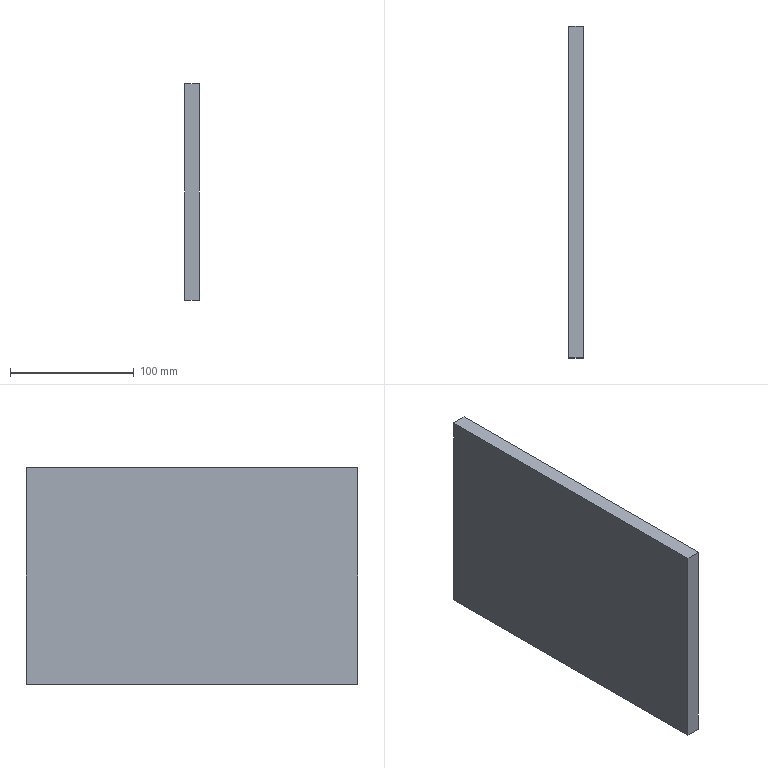Part | SolidWorks | features Extrusion 1 | 1 solid | 6 faces | box 12 x 268 x 175 mm | volume 562800 mm3 | plane 6
STEP:
#1=CARTESIAN_POINT('',(0.,268.,0.));
#2=VERTEX_POINT('',#1);
#3=CARTESIAN_POINT('',(0.,0.,0.));
#4=VERTEX_POINT('',#3);
#5=CARTESIAN_POINT('',(0.,0.,0.));
#6=DIRECTION('',(0.,-1.,0.));
#7=VECTOR('',#6,1000.);
#8=LINE('',#5,#7);
#9=EDGE_CURVE('',#2,#4,#8,.T.);
#10=ORIENTED_EDGE('',*,*,#9,.T.);
#11=CARTESIAN_POINT('',(12.,0.,0.));
#12=VERTEX_POINT('',#11);
#13=CARTESIAN_POINT('',(12.,0.,0.));
#14=DIRECTION('',(-1.,0.,0.));
#15=VECTOR('',#14,1000.);
#16=LINE('',#13,#15);
#17=EDGE_CURVE('',#12,#4,#16,.T.);
#18=ORIENTED_EDGE('',*,*,#17,.F.);
#19=CARTESIAN_POINT('',(12.,268.,0.));
#20=VERTEX_POINT('',#19);
#21=CARTESIAN_POINT('',(12.,0.,0.));
#22=DIRECTION('',(0.,-1.,0.));
#23=VECTOR('',#22,1000.);
#24=LINE('',#21,#23);
#25=EDGE_CURVE('',#20,#12,#24,.T.);
#26=ORIENTED_EDGE('',*,*,#25,.F.);
#27=CARTESIAN_POINT('',(12.,268.,0.));
#28=DIRECTION('',(-1.,0.,0.));
#29=VECTOR('',#28,1000.);
#30=LINE('',#27,#29);
#31=EDGE_CURVE('',#20,#2,#30,.T.);
#32=ORIENTED_EDGE('',*,*,#31,.T.);
#33=EDGE_LOOP('',(#10,#18,#26,#32));
#34=FACE_OUTER_BOUND('',#33,.T.);
#35=CARTESIAN_POINT('',(12.,0.,0.));
#36=DIRECTION('',(0.,0.,-1.));
#37=DIRECTION('',(-1.,0.,0.));
#38=AXIS2_PLACEMENT_3D('',#35,#36,#37);
#39=PLANE('',#38);
#40=ADVANCED_FACE('',(#34),#39,.F.);
#41=CARTESIAN_POINT('',(0.,0.,-175.));
#42=VERTEX_POINT('',#41);
#43=CARTESIAN_POINT('',(0.,0.,0.));
#44=DIRECTION('',(0.,0.,-1.));
#45=VECTOR('',#44,1000.);
#46=LINE('',#43,#45);
#47=EDGE_CURVE('',#4,#42,#46,.T.);
#48=ORIENTED_EDGE('',*,*,#47,.T.);
#49=CARTESIAN_POINT('',(12.,0.,-175.));
#50=VERTEX_POINT('',#49);
#51=CARTESIAN_POINT('',(12.,0.,-175.));
#52=DIRECTION('',(-1.,0.,0.));
#53=VECTOR('',#52,1000.);
#54=LINE('',#51,#53);
#55=EDGE_CURVE('',#50,#42,#54,.T.);
#56=ORIENTED_EDGE('',*,*,#55,.F.);
#57=CARTESIAN_POINT('',(12.,0.,0.));
#58=DIRECTION('',(0.,0.,-1.));
#59=VECTOR('',#58,1000.);
#60=LINE('',#57,#59);
#61=EDGE_CURVE('',#12,#50,#60,.T.);
#62=ORIENTED_EDGE('',*,*,#61,.F.);
#63=ORIENTED_EDGE('',*,*,#17,.T.);
#64=EDGE_LOOP('',(#48,#56,#62,#63));
#65=FACE_OUTER_BOUND('',#64,.T.);
#66=CARTESIAN_POINT('',(12.,0.,0.));
#67=DIRECTION('',(0.,1.,0.));
#68=DIRECTION('',(0.,0.,1.));
#69=AXIS2_PLACEMENT_3D('',#66,#67,#68);
#70=PLANE('',#69);
#71=ADVANCED_FACE('',(#65),#70,.F.);
#72=CARTESIAN_POINT('',(0.,268.,-175.));
#73=VERTEX_POINT('',#72);
#74=CARTESIAN_POINT('',(0.,0.,-175.));
#75=DIRECTION('',(0.,1.,0.));
#76=VECTOR('',#75,1000.);
#77=LINE('',#74,#76);
#78=EDGE_CURVE('',#42,#73,#77,.T.);
#79=ORIENTED_EDGE('',*,*,#78,.T.);
#80=CARTESIAN_POINT('',(12.,268.,-175.));
#81=VERTEX_POINT('',#80);
#82=CARTESIAN_POINT('',(12.,268.,-175.));
#83=DIRECTION('',(-1.,0.,0.));
#84=VECTOR('',#83,1000.);
#85=LINE('',#82,#84);
#86=EDGE_CURVE('',#81,#73,#85,.T.);
#87=ORIENTED_EDGE('',*,*,#86,.F.);
#88=CARTESIAN_POINT('',(12.,0.,-175.));
#89=DIRECTION('',(0.,1.,0.));
#90=VECTOR('',#89,1000.);
#91=LINE('',#88,#90);
#92=EDGE_CURVE('',#50,#81,#91,.T.);
#93=ORIENTED_EDGE('',*,*,#92,.F.);
#94=ORIENTED_EDGE('',*,*,#55,.T.);
#95=EDGE_LOOP('',(#79,#87,#93,#94));
#96=FACE_OUTER_BOUND('',#95,.T.);
#97=CARTESIAN_POINT('',(12.,0.,-175.));
#98=DIRECTION('',(0.,0.,1.));
#99=DIRECTION('',(1.,0.,0.));
#100=AXIS2_PLACEMENT_3D('',#97,#98,#99);
#101=PLANE('',#100);
#102=ADVANCED_FACE('',(#96),#101,.F.);
#103=CARTESIAN_POINT('',(0.,268.,0.));
#104=DIRECTION('',(0.,0.,1.));
#105=VECTOR('',#104,1000.);
#106=LINE('',#103,#105);
#107=EDGE_CURVE('',#73,#2,#106,.T.);
#108=ORIENTED_EDGE('',*,*,#107,.T.);
#109=ORIENTED_EDGE('',*,*,#31,.F.);
#110=CARTESIAN_POINT('',(12.,268.,0.));
#111=DIRECTION('',(0.,0.,1.));
#112=VECTOR('',#111,1000.);
#113=LINE('',#110,#112);
#114=EDGE_CURVE('',#81,#20,#113,.T.);
#115=ORIENTED_EDGE('',*,*,#114,.F.);
#116=ORIENTED_EDGE('',*,*,#86,.T.);
#117=EDGE_LOOP('',(#108,#109,#115,#116));
#118=FACE_OUTER_BOUND('',#117,.T.);
#119=CARTESIAN_POINT('',(12.,268.,0.));
#120=DIRECTION('',(0.,-1.,0.));
#121=DIRECTION('',(0.,0.,-1.));
#122=AXIS2_PLACEMENT_3D('',#119,#120,#121);
#123=PLANE('',#122);
#124=ADVANCED_FACE('',(#118),#123,.F.);
#125=ORIENTED_EDGE('',*,*,#25,.T.);
#126=ORIENTED_EDGE('',*,*,#61,.T.);
#127=ORIENTED_EDGE('',*,*,#92,.T.);
#128=ORIENTED_EDGE('',*,*,#114,.T.);
#129=EDGE_LOOP('',(#125,#126,#127,#128));
#130=FACE_OUTER_BOUND('',#129,.T.);
#131=CARTESIAN_POINT('',(12.,268.,0.));
#132=DIRECTION('',(-1.,0.,0.));
#133=DIRECTION('',(0.,0.,1.));
#134=AXIS2_PLACEMENT_3D('',#131,#132,#133);
#135=PLANE('',#134);
#136=ADVANCED_FACE('',(#130),#135,.F.);
#137=ORIENTED_EDGE('',*,*,#9,.F.);
#138=ORIENTED_EDGE('',*,*,#107,.F.);
#139=ORIENTED_EDGE('',*,*,#78,.F.);
#140=ORIENTED_EDGE('',*,*,#47,.F.);
#141=EDGE_LOOP('',(#137,#138,#139,#140));
#142=FACE_OUTER_BOUND('',#141,.T.);
#143=CARTESIAN_POINT('',(0.,268.,0.));
#144=DIRECTION('',(-1.,0.,0.));
#145=DIRECTION('',(0.,0.,1.));
#146=AXIS2_PLACEMENT_3D('',#143,#144,#145);
#147=PLANE('',#146);
#148=ADVANCED_FACE('',(#142),#147,.T.);
#149=CLOSED_SHELL('',(#40,#71,#102,#124,#136,#148));
#150=MANIFOLD_SOLID_BREP('',#149);
#151=CARTESIAN_POINT('',(0.,0.,0.));
#152=DIRECTION('',(0.,0.,1.));
#153=DIRECTION('',(1.,0.,0.));
#154=AXIS2_PLACEMENT_3D('',#151,#152,#153);
#155=(LENGTH_UNIT()NAMED_UNIT(*)SI_UNIT(.MILLI.,.METRE.));
#156=UNCERTAINTY_MEASURE_WITH_UNIT(LENGTH_MEASURE(0.00001),#155,'','');
#157=(NAMED_UNIT(*)PLANE_ANGLE_UNIT()SI_UNIT($,.RADIAN.));
#158=(NAMED_UNIT(*)SI_UNIT($,.STERADIAN.)SOLID_ANGLE_UNIT());
#159=(GEOMETRIC_REPRESENTATION_CONTEXT(3)GLOBAL_UNCERTAINTY_ASSIGNED_CONTEXT((#156))GLOBAL_UNIT_ASSIGNED_CONTEXT((#155,#157,#158))REPRESENTATION_CONTEXT('',''));
#160=ADVANCED_BREP_SHAPE_REPRESENTATION('',(#150,#154),#159);